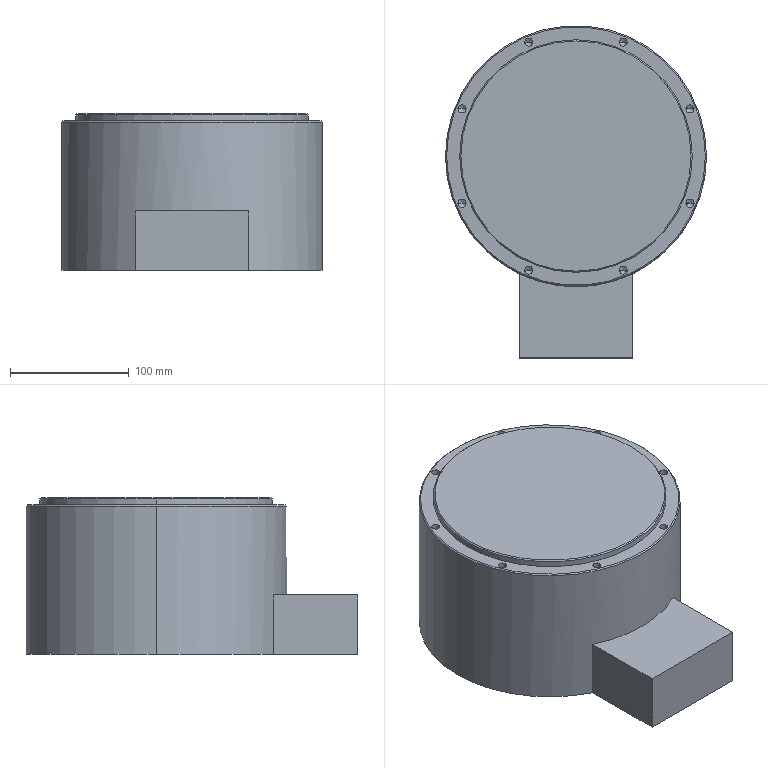Part | SolidWorks | features ICE 3, HoleWzd 2, Chamfer 1, Extrusion 1 | 1 solid | 51 faces | box 220 x 280 x 132 mm | volume 5270388 mm3 | cylinder 22 | cone 22 | plane 7 | commonest cylinder face diameters 6.8 x18 196 x2 220 x2
STEP:
#1=CARTESIAN_POINT('',(36.399,96.083,112.25));
#2=VERTEX_POINT('',#1);
#3=CARTESIAN_POINT('',(43.199,96.083,112.25));
#4=VERTEX_POINT('',#3);
#5=CARTESIAN_POINT('',(39.799,96.083,112.25));
#6=DIRECTION('',(0.,0.,1.));
#7=DIRECTION('',(1.,0.,0.));
#8=AXIS2_PLACEMENT_3D('',#5,#6,#7);
#9=CIRCLE('',#8,3.4);
#10=EDGE_CURVE('',#2,#4,#9,.T.);
#11=ORIENTED_EDGE('',*,*,#10,.F.);
#12=CARTESIAN_POINT('',(36.399,96.083,126.));
#13=VERTEX_POINT('',#12);
#14=CARTESIAN_POINT('',(36.399,96.083,132.));
#15=DIRECTION('',(0.,0.,1.));
#16=VECTOR('',#15,1000.);
#17=LINE('',#14,#16);
#18=EDGE_CURVE('',#2,#13,#17,.T.);
#19=ORIENTED_EDGE('',*,*,#18,.T.);
#20=CARTESIAN_POINT('',(43.199,96.083,126.));
#21=VERTEX_POINT('',#20);
#22=CARTESIAN_POINT('',(39.799,96.083,126.));
#23=DIRECTION('',(0.,0.,1.));
#24=DIRECTION('',(1.,0.,0.));
#25=AXIS2_PLACEMENT_3D('',#22,#23,#24);
#26=CIRCLE('',#25,3.4);
#27=EDGE_CURVE('',#13,#21,#26,.T.);
#28=ORIENTED_EDGE('',*,*,#27,.T.);
#29=CARTESIAN_POINT('',(43.199,96.083,132.));
#30=DIRECTION('',(0.,0.,1.));
#31=VECTOR('',#30,1000.);
#32=LINE('',#29,#31);
#33=EDGE_CURVE('',#4,#21,#32,.T.);
#34=ORIENTED_EDGE('',*,*,#33,.F.);
#35=EDGE_LOOP('',(#11,#19,#28,#34));
#36=FACE_OUTER_BOUND('',#35,.T.);
#37=CARTESIAN_POINT('',(39.799,96.083,132.));
#38=DIRECTION('',(0.,0.,1.));
#39=DIRECTION('',(1.,0.,0.));
#40=AXIS2_PLACEMENT_3D('',#37,#38,#39);
#41=CYLINDRICAL_SURFACE('',#40,3.4);
#42=ADVANCED_FACE('',(#36),#41,.F.);
#43=CARTESIAN_POINT('',(39.799,96.083,110.207));
#44=VERTEX_POINT('',#43);
#45=CARTESIAN_POINT('',(43.199,96.083,112.25));
#46=DIRECTION('',(0.8572,0.,0.515));
#47=VECTOR('',#46,1000.);
#48=LINE('',#45,#47);
#49=EDGE_CURVE('',#44,#4,#48,.T.);
#50=ORIENTED_EDGE('',*,*,#49,.F.);
#51=CARTESIAN_POINT('',(36.399,96.083,112.25));
#52=DIRECTION('',(-0.8572,0.,0.515));
#53=VECTOR('',#52,1000.);
#54=LINE('',#51,#53);
#55=EDGE_CURVE('',#44,#2,#54,.T.);
#56=ORIENTED_EDGE('',*,*,#55,.T.);
#57=ORIENTED_EDGE('',*,*,#10,.T.);
#58=EDGE_LOOP('',(#50,#56,#57));
#59=FACE_OUTER_BOUND('',#58,.T.);
#60=CARTESIAN_POINT('',(39.799,96.083,112.25));
#61=DIRECTION('',(0.,0.,1.));
#62=DIRECTION('',(1.,0.,0.));
#63=AXIS2_PLACEMENT_3D('',#60,#61,#62);
#64=CONICAL_SURFACE('',#63,3.4,1.03);
#65=ADVANCED_FACE('',(#59),#64,.F.);
#66=CARTESIAN_POINT('',(92.683,39.799,112.25));
#67=VERTEX_POINT('',#66);
#68=CARTESIAN_POINT('',(99.483,39.799,112.25));
#69=VERTEX_POINT('',#68);
#70=CARTESIAN_POINT('',(96.083,39.799,112.25));
#71=DIRECTION('',(0.,0.,1.));
#72=DIRECTION('',(1.,0.,0.));
#73=AXIS2_PLACEMENT_3D('',#70,#71,#72);
#74=CIRCLE('',#73,3.4);
#75=EDGE_CURVE('',#67,#69,#74,.T.);
#76=ORIENTED_EDGE('',*,*,#75,.F.);
#77=CARTESIAN_POINT('',(92.683,39.799,126.));
#78=VERTEX_POINT('',#77);
#79=CARTESIAN_POINT('',(92.683,39.799,132.));
#80=DIRECTION('',(0.,0.,1.));
#81=VECTOR('',#80,1000.);
#82=LINE('',#79,#81);
#83=EDGE_CURVE('',#67,#78,#82,.T.);
#84=ORIENTED_EDGE('',*,*,#83,.T.);
#85=CARTESIAN_POINT('',(99.483,39.799,126.));
#86=VERTEX_POINT('',#85);
#87=CARTESIAN_POINT('',(96.083,39.799,126.));
#88=DIRECTION('',(0.,0.,1.));
#89=DIRECTION('',(1.,0.,0.));
#90=AXIS2_PLACEMENT_3D('',#87,#88,#89);
#91=CIRCLE('',#90,3.4);
#92=EDGE_CURVE('',#78,#86,#91,.T.);
#93=ORIENTED_EDGE('',*,*,#92,.T.);
#94=CARTESIAN_POINT('',(99.483,39.799,132.));
#95=DIRECTION('',(0.,0.,1.));
#96=VECTOR('',#95,1000.);
#97=LINE('',#94,#96);
#98=EDGE_CURVE('',#69,#86,#97,.T.);
#99=ORIENTED_EDGE('',*,*,#98,.F.);
#100=EDGE_LOOP('',(#76,#84,#93,#99));
#101=FACE_OUTER_BOUND('',#100,.T.);
#102=CARTESIAN_POINT('',(96.083,39.799,132.));
#103=DIRECTION('',(0.,0.,1.));
#104=DIRECTION('',(1.,0.,0.));
#105=AXIS2_PLACEMENT_3D('',#102,#103,#104);
#106=CYLINDRICAL_SURFACE('',#105,3.4);
#107=ADVANCED_FACE('',(#101),#106,.F.);
#108=CARTESIAN_POINT('',(96.083,39.799,110.207));
#109=VERTEX_POINT('',#108);
#110=CARTESIAN_POINT('',(99.483,39.799,112.25));
#111=DIRECTION('',(0.8572,0.,0.515));
#112=VECTOR('',#111,1000.);
#113=LINE('',#110,#112);
#114=EDGE_CURVE('',#109,#69,#113,.T.);
#115=ORIENTED_EDGE('',*,*,#114,.F.);
#116=CARTESIAN_POINT('',(92.683,39.799,112.25));
#117=DIRECTION('',(-0.8572,0.,0.515));
#118=VECTOR('',#117,1000.);
#119=LINE('',#116,#118);
#120=EDGE_CURVE('',#109,#67,#119,.T.);
#121=ORIENTED_EDGE('',*,*,#120,.T.);
#122=ORIENTED_EDGE('',*,*,#75,.T.);
#123=EDGE_LOOP('',(#115,#121,#122));
#124=FACE_OUTER_BOUND('',#123,.T.);
#125=CARTESIAN_POINT('',(96.083,39.799,112.25));
#126=DIRECTION('',(0.,0.,1.));
#127=DIRECTION('',(1.,0.,0.));
#128=AXIS2_PLACEMENT_3D('',#125,#126,#127);
#129=CONICAL_SURFACE('',#128,3.4,1.03);
#130=ADVANCED_FACE('',(#124),#129,.F.);
#131=CARTESIAN_POINT('',(92.683,-39.799,112.25));
#132=VERTEX_POINT('',#131);
#133=CARTESIAN_POINT('',(99.483,-39.799,112.25));
#134=VERTEX_POINT('',#133);
#135=CARTESIAN_POINT('',(96.083,-39.799,112.25));
#136=DIRECTION('',(0.,0.,1.));
#137=DIRECTION('',(1.,0.,0.));
#138=AXIS2_PLACEMENT_3D('',#135,#136,#137);
#139=CIRCLE('',#138,3.4);
#140=EDGE_CURVE('',#132,#134,#139,.T.);
#141=ORIENTED_EDGE('',*,*,#140,.F.);
#142=CARTESIAN_POINT('',(92.683,-39.799,126.));
#143=VERTEX_POINT('',#142);
#144=CARTESIAN_POINT('',(92.683,-39.799,132.));
#145=DIRECTION('',(0.,0.,1.));
#146=VECTOR('',#145,1000.);
#147=LINE('',#144,#146);
#148=EDGE_CURVE('',#132,#143,#147,.T.);
#149=ORIENTED_EDGE('',*,*,#148,.T.);
#150=CARTESIAN_POINT('',(99.483,-39.799,126.));
#151=VERTEX_POINT('',#150);
#152=CARTESIAN_POINT('',(96.083,-39.799,126.));
#153=DIRECTION('',(0.,0.,1.));
#154=DIRECTION('',(1.,0.,0.));
#155=AXIS2_PLACEMENT_3D('',#152,#153,#154);
#156=CIRCLE('',#155,3.4);
#157=EDGE_CURVE('',#143,#151,#156,.T.);
#158=ORIENTED_EDGE('',*,*,#157,.T.);
#159=CARTESIAN_POINT('',(99.483,-39.799,132.));
#160=DIRECTION('',(0.,0.,1.));
#161=VECTOR('',#160,1000.);
#162=LINE('',#159,#161);
#163=EDGE_CURVE('',#134,#151,#162,.T.);
#164=ORIENTED_EDGE('',*,*,#163,.F.);
#165=EDGE_LOOP('',(#141,#149,#158,#164));
#166=FACE_OUTER_BOUND('',#165,.T.);
#167=CARTESIAN_POINT('',(96.083,-39.799,132.));
#168=DIRECTION('',(0.,0.,1.));
#169=DIRECTION('',(1.,0.,0.));
#170=AXIS2_PLACEMENT_3D('',#167,#168,#169);
#171=CYLINDRICAL_SURFACE('',#170,3.4);
#172=ADVANCED_FACE('',(#166),#171,.F.);
#173=CARTESIAN_POINT('',(96.083,-39.799,110.207));
#174=VERTEX_POINT('',#173);
#175=CARTESIAN_POINT('',(99.483,-39.799,112.25));
#176=DIRECTION('',(0.8572,0.,0.515));
#177=VECTOR('',#176,1000.);
#178=LINE('',#175,#177);
#179=EDGE_CURVE('',#174,#134,#178,.T.);
#180=ORIENTED_EDGE('',*,*,#179,.F.);
#181=CARTESIAN_POINT('',(92.683,-39.799,112.25));
#182=DIRECTION('',(-0.8572,0.,0.515));
#183=VECTOR('',#182,1000.);
#184=LINE('',#181,#183);
#185=EDGE_CURVE('',#174,#132,#184,.T.);
#186=ORIENTED_EDGE('',*,*,#185,.T.);
#187=ORIENTED_EDGE('',*,*,#140,.T.);
#188=EDGE_LOOP('',(#180,#186,#187));
#189=FACE_OUTER_BOUND('',#188,.T.);
#190=CARTESIAN_POINT('',(96.083,-39.799,112.25));
#191=DIRECTION('',(0.,0.,1.));
#192=DIRECTION('',(1.,0.,0.));
#193=AXIS2_PLACEMENT_3D('',#190,#191,#192);
#194=CONICAL_SURFACE('',#193,3.4,1.03);
#195=ADVANCED_FACE('',(#189),#194,.F.);
#196=CARTESIAN_POINT('',(36.399,-96.083,112.25));
#197=VERTEX_POINT('',#196);
#198=CARTESIAN_POINT('',(43.199,-96.083,112.25));
#199=VERTEX_POINT('',#198);
#200=CARTESIAN_POINT('',(39.799,-96.083,112.25));
#201=DIRECTION('',(0.,0.,1.));
#202=DIRECTION('',(1.,0.,0.));
#203=AXIS2_PLACEMENT_3D('',#200,#201,#202);
#204=CIRCLE('',#203,3.4);
#205=EDGE_CURVE('',#197,#199,#204,.T.);
#206=ORIENTED_EDGE('',*,*,#205,.F.);
#207=CARTESIAN_POINT('',(36.399,-96.083,126.));
#208=VERTEX_POINT('',#207);
#209=CARTESIAN_POINT('',(36.399,-96.083,132.));
#210=DIRECTION('',(0.,0.,1.));
#211=VECTOR('',#210,1000.);
#212=LINE('',#209,#211);
#213=EDGE_CURVE('',#197,#208,#212,.T.);
#214=ORIENTED_EDGE('',*,*,#213,.T.);
#215=CARTESIAN_POINT('',(43.199,-96.083,126.));
#216=VERTEX_POINT('',#215);
#217=CARTESIAN_POINT('',(39.799,-96.083,126.));
#218=DIRECTION('',(0.,0.,1.));
#219=DIRECTION('',(1.,0.,0.));
#220=AXIS2_PLACEMENT_3D('',#217,#218,#219);
#221=CIRCLE('',#220,3.4);
#222=EDGE_CURVE('',#208,#216,#221,.T.);
#223=ORIENTED_EDGE('',*,*,#222,.T.);
#224=CARTESIAN_POINT('',(43.199,-96.083,132.));
#225=DIRECTION('',(0.,0.,1.));
#226=VECTOR('',#225,1000.);
#227=LINE('',#224,#226);
#228=EDGE_CURVE('',#199,#216,#227,.T.);
#229=ORIENTED_EDGE('',*,*,#228,.F.);
#230=EDGE_LOOP('',(#206,#214,#223,#229));
#231=FACE_OUTER_BOUND('',#230,.T.);
#232=CARTESIAN_POINT('',(39.799,-96.083,132.));
#233=DIRECTION('',(0.,0.,1.));
#234=DIRECTION('',(1.,0.,0.));
#235=AXIS2_PLACEMENT_3D('',#232,#233,#234);
#236=CYLINDRICAL_SURFACE('',#235,3.4);
#237=ADVANCED_FACE('',(#231),#236,.F.);
#238=CARTESIAN_POINT('',(39.799,-96.083,110.207));
#239=VERTEX_POINT('',#238);
#240=CARTESIAN_POINT('',(43.199,-96.083,112.25));
#241=DIRECTION('',(0.8572,0.,0.515));
#242=VECTOR('',#241,1000.);
#243=LINE('',#240,#242);
#244=EDGE_CURVE('',#239,#199,#243,.T.);
#245=ORIENTED_EDGE('',*,*,#244,.F.);
#246=CARTESIAN_POINT('',(36.399,-96.083,112.25));
#247=DIRECTION('',(-0.8572,0.,0.515));
#248=VECTOR('',#247,1000.);
#249=LINE('',#246,#248);
#250=EDGE_CURVE('',#239,#197,#249,.T.);
#251=ORIENTED_EDGE('',*,*,#250,.T.);
#252=ORIENTED_EDGE('',*,*,#205,.T.);
#253=EDGE_LOOP('',(#245,#251,#252));
#254=FACE_OUTER_BOUND('',#253,.T.);
#255=CARTESIAN_POINT('',(39.799,-96.083,112.25));
#256=DIRECTION('',(0.,0.,1.));
#257=DIRECTION('',(1.,0.,0.));
#258=AXIS2_PLACEMENT_3D('',#255,#256,#257);
#259=CONICAL_SURFACE('',#258,3.4,1.03);
#260=ADVANCED_FACE('',(#254),#259,.F.);
#261=CARTESIAN_POINT('',(-43.199,-96.083,112.25));
#262=VERTEX_POINT('',#261);
#263=CARTESIAN_POINT('',(-36.399,-96.083,112.25));
#264=VERTEX_POINT('',#263);
#265=CARTESIAN_POINT('',(-39.799,-96.083,112.25));
#266=DIRECTION('',(0.,0.,1.));
#267=DIRECTION('',(1.,0.,0.));
#268=AXIS2_PLACEMENT_3D('',#265,#266,#267);
#269=CIRCLE('',#268,3.4);
#270=EDGE_CURVE('',#262,#264,#269,.T.);
#271=ORIENTED_EDGE('',*,*,#270,.F.);
#272=CARTESIAN_POINT('',(-43.199,-96.083,126.));
#273=VERTEX_POINT('',#272);
#274=CARTESIAN_POINT('',(-43.199,-96.083,132.));
#275=DIRECTION('',(0.,0.,1.));
#276=VECTOR('',#275,1000.);
#277=LINE('',#274,#276);
#278=EDGE_CURVE('',#262,#273,#277,.T.);
#279=ORIENTED_EDGE('',*,*,#278,.T.);
#280=CARTESIAN_POINT('',(-36.399,-96.083,126.));
#281=VERTEX_POINT('',#280);
#282=CARTESIAN_POINT('',(-39.799,-96.083,126.));
#283=DIRECTION('',(0.,0.,1.));
#284=DIRECTION('',(1.,0.,0.));
#285=AXIS2_PLACEMENT_3D('',#282,#283,#284);
#286=CIRCLE('',#285,3.4);
#287=EDGE_CURVE('',#273,#281,#286,.T.);
#288=ORIENTED_EDGE('',*,*,#287,.T.);
#289=CARTESIAN_POINT('',(-36.399,-96.083,132.));
#290=DIRECTION('',(0.,0.,1.));
#291=VECTOR('',#290,1000.);
#292=LINE('',#289,#291);
#293=EDGE_CURVE('',#264,#281,#292,.T.);
#294=ORIENTED_EDGE('',*,*,#293,.F.);
#295=EDGE_LOOP('',(#271,#279,#288,#294));
#296=FACE_OUTER_BOUND('',#295,.T.);
#297=CARTESIAN_POINT('',(-39.799,-96.083,132.));
#298=DIRECTION('',(0.,0.,1.));
#299=DIRECTION('',(1.,0.,0.));
#300=AXIS2_PLACEMENT_3D('',#297,#298,#299);
#301=CYLINDRICAL_SURFACE('',#300,3.4);
#302=ADVANCED_FACE('',(#296),#301,.F.);
#303=CARTESIAN_POINT('',(-39.799,-96.083,110.207));
#304=VERTEX_POINT('',#303);
#305=CARTESIAN_POINT('',(-36.399,-96.083,112.25));
#306=DIRECTION('',(0.8572,0.,0.515));
#307=VECTOR('',#306,1000.);
#308=LINE('',#305,#307);
#309=EDGE_CURVE('',#304,#264,#308,.T.);
#310=ORIENTED_EDGE('',*,*,#309,.F.);
#311=CARTESIAN_POINT('',(-43.199,-96.083,112.25));
#312=DIRECTION('',(-0.8572,0.,0.515));
#313=VECTOR('',#312,1000.);
#314=LINE('',#311,#313);
#315=EDGE_CURVE('',#304,#262,#314,.T.);
#316=ORIENTED_EDGE('',*,*,#315,.T.);
#317=ORIENTED_EDGE('',*,*,#270,.T.);
#318=EDGE_LOOP('',(#310,#316,#317));
#319=FACE_OUTER_BOUND('',#318,.T.);
#320=CARTESIAN_POINT('',(-39.799,-96.083,112.25));
#321=DIRECTION('',(0.,0.,1.));
#322=DIRECTION('',(1.,0.,0.));
#323=AXIS2_PLACEMENT_3D('',#320,#321,#322);
#324=CONICAL_SURFACE('',#323,3.4,1.03);
#325=ADVANCED_FACE('',(#319),#324,.F.);
#326=CARTESIAN_POINT('',(-99.483,-39.799,112.25));
#327=VERTEX_POINT('',#326);
#328=CARTESIAN_POINT('',(-92.683,-39.799,112.25));
#329=VERTEX_POINT('',#328);
#330=CARTESIAN_POINT('',(-96.083,-39.799,112.25));
#331=DIRECTION('',(0.,0.,1.));
#332=DIRECTION('',(1.,0.,0.));
#333=AXIS2_PLACEMENT_3D('',#330,#331,#332);
#334=CIRCLE('',#333,3.4);
#335=EDGE_CURVE('',#327,#329,#334,.T.);
#336=ORIENTED_EDGE('',*,*,#335,.F.);
#337=CARTESIAN_POINT('',(-99.483,-39.799,126.));
#338=VERTEX_POINT('',#337);
#339=CARTESIAN_POINT('',(-99.483,-39.799,132.));
#340=DIRECTION('',(0.,0.,1.));
#341=VECTOR('',#340,1000.);
#342=LINE('',#339,#341);
#343=EDGE_CURVE('',#327,#338,#342,.T.);
#344=ORIENTED_EDGE('',*,*,#343,.T.);
#345=CARTESIAN_POINT('',(-92.683,-39.799,126.));
#346=VERTEX_POINT('',#345);
#347=CARTESIAN_POINT('',(-96.083,-39.799,126.));
#348=DIRECTION('',(0.,0.,1.));
#349=DIRECTION('',(1.,0.,0.));
#350=AXIS2_PLACEMENT_3D('',#347,#348,#349);
#351=CIRCLE('',#350,3.4);
#352=EDGE_CURVE('',#338,#346,#351,.T.);
#353=ORIENTED_EDGE('',*,*,#352,.T.);
#354=CARTESIAN_POINT('',(-92.683,-39.799,132.));
#355=DIRECTION('',(0.,0.,1.));
#356=VECTOR('',#355,1000.);
#357=LINE('',#354,#356);
#358=EDGE_CURVE('',#329,#346,#357,.T.);
#359=ORIENTED_EDGE('',*,*,#358,.F.);
#360=EDGE_LOOP('',(#336,#344,#353,#359));
#361=FACE_OUTER_BOUND('',#360,.T.);
#362=CARTESIAN_POINT('',(-96.083,-39.799,132.));
#363=DIRECTION('',(0.,0.,1.));
#364=DIRECTION('',(1.,0.,0.));
#365=AXIS2_PLACEMENT_3D('',#362,#363,#364);
#366=CYLINDRICAL_SURFACE('',#365,3.4);
#367=ADVANCED_FACE('',(#361),#366,.F.);
#368=CARTESIAN_POINT('',(-96.083,-39.799,110.207));
#369=VERTEX_POINT('',#368);
#370=CARTESIAN_POINT('',(-92.683,-39.799,112.25));
#371=DIRECTION('',(0.8572,0.,0.515));
#372=VECTOR('',#371,1000.);
#373=LINE('',#370,#372);
#374=EDGE_CURVE('',#369,#329,#373,.T.);
#375=ORIENTED_EDGE('',*,*,#374,.F.);
#376=CARTESIAN_POINT('',(-99.483,-39.799,112.25));
#377=DIRECTION('',(-0.8572,0.,0.515));
#378=VECTOR('',#377,1000.);
#379=LINE('',#376,#378);
#380=EDGE_CURVE('',#369,#327,#379,.T.);
#381=ORIENTED_EDGE('',*,*,#380,.T.);
#382=ORIENTED_EDGE('',*,*,#335,.T.);
#383=EDGE_LOOP('',(#375,#381,#382));
#384=FACE_OUTER_BOUND('',#383,.T.);
#385=CARTESIAN_POINT('',(-96.083,-39.799,112.25));
#386=DIRECTION('',(0.,0.,1.));
#387=DIRECTION('',(1.,0.,0.));
#388=AXIS2_PLACEMENT_3D('',#385,#386,#387);
#389=CONICAL_SURFACE('',#388,3.4,1.03);
#390=ADVANCED_FACE('',(#384),#389,.F.);
#391=CARTESIAN_POINT('',(-99.483,39.799,112.25));
#392=VERTEX_POINT('',#391);
#393=CARTESIAN_POINT('',(-92.683,39.799,112.25));
#394=VERTEX_POINT('',#393);
#395=CARTESIAN_POINT('',(-96.083,39.799,112.25));
#396=DIRECTION('',(0.,0.,1.));
#397=DIRECTION('',(1.,0.,0.));
#398=AXIS2_PLACEMENT_3D('',#395,#396,#397);
#399=CIRCLE('',#398,3.4);
#400=EDGE_CURVE('',#392,#394,#399,.T.);
#401=ORIENTED_EDGE('',*,*,#400,.F.);
#402=CARTESIAN_POINT('',(-99.483,39.799,126.));
#403=VERTEX_POINT('',#402);
#404=CARTESIAN_POINT('',(-99.483,39.799,132.));
#405=DIRECTION('',(0.,0.,1.));
#406=VECTOR('',#405,1000.);
#407=LINE('',#404,#406);
#408=EDGE_CURVE('',#392,#403,#407,.T.);
#409=ORIENTED_EDGE('',*,*,#408,.T.);
#410=CARTESIAN_POINT('',(-92.683,39.799,126.));
#411=VERTEX_POINT('',#410);
#412=CARTESIAN_POINT('',(-96.083,39.799,126.));
#413=DIRECTION('',(0.,0.,1.));
#414=DIRECTION('',(1.,0.,0.));
#415=AXIS2_PLACEMENT_3D('',#412,#413,#414);
#416=CIRCLE('',#415,3.4);
#417=EDGE_CURVE('',#403,#411,#416,.T.);
#418=ORIENTED_EDGE('',*,*,#417,.T.);
#419=CARTESIAN_POINT('',(-92.683,39.799,132.));
#420=DIRECTION('',(0.,0.,1.));
#421=VECTOR('',#420,1000.);
#422=LINE('',#419,#421);
#423=EDGE_CURVE('',#394,#411,#422,.T.);
#424=ORIENTED_EDGE('',*,*,#423,.F.);
#425=EDGE_LOOP('',(#401,#409,#418,#424));
#426=FACE_OUTER_BOUND('',#425,.T.);
#427=CARTESIAN_POINT('',(-96.083,39.799,132.));
#428=DIRECTION('',(0.,0.,1.));
#429=DIRECTION('',(1.,0.,0.));
#430=AXIS2_PLACEMENT_3D('',#427,#428,#429);
#431=CYLINDRICAL_SURFACE('',#430,3.4);
#432=ADVANCED_FACE('',(#426),#431,.F.);
#433=CARTESIAN_POINT('',(-96.083,39.799,110.207));
#434=VERTEX_POINT('',#433);
#435=CARTESIAN_POINT('',(-92.683,39.799,112.25));
#436=DIRECTION('',(0.8572,0.,0.515));
#437=VECTOR('',#436,1000.);
#438=LINE('',#435,#437);
#439=EDGE_CURVE('',#434,#394,#438,.T.);
#440=ORIENTED_EDGE('',*,*,#439,.F.);
#441=CARTESIAN_POINT('',(-99.483,39.799,112.25));
#442=DIRECTION('',(-0.8572,0.,0.515));
#443=VECTOR('',#442,1000.);
#444=LINE('',#441,#443);
#445=EDGE_CURVE('',#434,#392,#444,.T.);
#446=ORIENTED_EDGE('',*,*,#445,.T.);
#447=ORIENTED_EDGE('',*,*,#400,.T.);
#448=EDGE_LOOP('',(#440,#446,#447));
#449=FACE_OUTER_BOUND('',#448,.T.);
#450=CARTESIAN_POINT('',(-96.083,39.799,112.25));
#451=DIRECTION('',(0.,0.,1.));
#452=DIRECTION('',(1.,0.,0.));
#453=AXIS2_PLACEMENT_3D('',#450,#451,#452);
#454=CONICAL_SURFACE('',#453,3.4,1.03);
#455=ADVANCED_FACE('',(#449),#454,.F.);
#456=CARTESIAN_POINT('',(-43.199,96.083,112.25));
#457=VERTEX_POINT('',#456);
#458=CARTESIAN_POINT('',(-36.399,96.083,112.25));
#459=VERTEX_POINT('',#458);
#460=CARTESIAN_POINT('',(-39.799,96.083,112.25));
#461=DIRECTION('',(0.,0.,1.));
#462=DIRECTION('',(1.,0.,0.));
#463=AXIS2_PLACEMENT_3D('',#460,#461,#462);
#464=CIRCLE('',#463,3.4);
#465=EDGE_CURVE('',#457,#459,#464,.T.);
#466=ORIENTED_EDGE('',*,*,#465,.F.);
#467=CARTESIAN_POINT('',(-43.199,96.083,126.));
#468=VERTEX_POINT('',#467);
#469=CARTESIAN_POINT('',(-43.199,96.083,132.));
#470=DIRECTION('',(0.,0.,1.));
#471=VECTOR('',#470,1000.);
#472=LINE('',#469,#471);
#473=EDGE_CURVE('',#457,#468,#472,.T.);
#474=ORIENTED_EDGE('',*,*,#473,.T.);
#475=CARTESIAN_POINT('',(-36.399,96.083,126.));
#476=VERTEX_POINT('',#475);
#477=CARTESIAN_POINT('',(-39.799,96.083,126.));
#478=DIRECTION('',(0.,0.,1.));
#479=DIRECTION('',(1.,0.,0.));
#480=AXIS2_PLACEMENT_3D('',#477,#478,#479);
#481=CIRCLE('',#480,3.4);
#482=EDGE_CURVE('',#468,#476,#481,.T.);
#483=ORIENTED_EDGE('',*,*,#482,.T.);
#484=CARTESIAN_POINT('',(-36.399,96.083,132.));
#485=DIRECTION('',(0.,0.,1.));
#486=VECTOR('',#485,1000.);
#487=LINE('',#484,#486);
#488=EDGE_CURVE('',#459,#476,#487,.T.);
#489=ORIENTED_EDGE('',*,*,#488,.F.);
#490=EDGE_LOOP('',(#466,#474,#483,#489));
#491=FACE_OUTER_BOUND('',#490,.T.);
#492=CARTESIAN_POINT('',(-39.799,96.083,132.));
#493=DIRECTION('',(0.,0.,1.));
#494=DIRECTION('',(1.,0.,0.));
#495=AXIS2_PLACEMENT_3D('',#492,#493,#494);
#496=CYLINDRICAL_SURFACE('',#495,3.4);
#497=ADVANCED_FACE('',(#491),#496,.F.);
#498=CARTESIAN_POINT('',(-39.799,96.083,110.207));
#499=VERTEX_POINT('',#498);
#500=CARTESIAN_POINT('',(-36.399,96.083,112.25));
#501=DIRECTION('',(0.8572,0.,0.515));
#502=VECTOR('',#501,1000.);
#503=LINE('',#500,#502);
#504=EDGE_CURVE('',#499,#459,#503,.T.);
#505=ORIENTED_EDGE('',*,*,#504,.F.);
#506=CARTESIAN_POINT('',(-43.199,96.083,112.25));
#507=DIRECTION('',(-0.8572,0.,0.515));
#508=VECTOR('',#507,1000.);
#509=LINE('',#506,#508);
#510=EDGE_CURVE('',#499,#457,#509,.T.);
#511=ORIENTED_EDGE('',*,*,#510,.T.);
#512=ORIENTED_EDGE('',*,*,#465,.T.);
#513=EDGE_LOOP('',(#505,#511,#512));
#514=FACE_OUTER_BOUND('',#513,.T.);
#515=CARTESIAN_POINT('',(-39.799,96.083,112.25));
#516=DIRECTION('',(0.,0.,1.));
#517=DIRECTION('',(1.,0.,0.));
#518=AXIS2_PLACEMENT_3D('',#515,#516,#517);
#519=CONICAL_SURFACE('',#518,3.4,1.03);
#520=ADVANCED_FACE('',(#514),#519,.F.);
#521=CARTESIAN_POINT('',(3.4,-115.,19.75));
#522=VERTEX_POINT('',#521);
#523=CARTESIAN_POINT('',(-3.4,-115.,19.75));
#524=VERTEX_POINT('',#523);
#525=CARTESIAN_POINT('',(0.,-115.,19.75));
#526=DIRECTION('',(0.,0.,-1.));
#527=DIRECTION('',(-1.,0.,0.));
#528=AXIS2_PLACEMENT_3D('',#525,#526,#527);
#529=CIRCLE('',#528,3.4);
#530=EDGE_CURVE('',#522,#524,#529,.T.);
#531=ORIENTED_EDGE('',*,*,#530,.F.);
#532=CARTESIAN_POINT('',(3.4,-115.,0.));
#533=VERTEX_POINT('',#532);
#534=CARTESIAN_POINT('',(3.4,-115.,0.));
#535=DIRECTION('',(0.,0.,-1.));
#536=VECTOR('',#535,1000.);
#537=LINE('',#534,#536);
#538=EDGE_CURVE('',#522,#533,#537,.T.);
#539=ORIENTED_EDGE('',*,*,#538,.T.);
#540=CARTESIAN_POINT('',(-3.4,-115.,0.));
#541=VERTEX_POINT('',#540);
#542=CARTESIAN_POINT('',(0.,-115.,0.));
#543=DIRECTION('',(0.,0.,-1.));
#544=DIRECTION('',(-1.,0.,0.));
#545=AXIS2_PLACEMENT_3D('',#542,#543,#544);
#546=CIRCLE('',#545,3.4);
#547=EDGE_CURVE('',#533,#541,#546,.T.);
#548=ORIENTED_EDGE('',*,*,#547,.T.);
#549=CARTESIAN_POINT('',(-3.4,-115.,0.));
#550=DIRECTION('',(0.,0.,-1.));
#551=VECTOR('',#550,1000.);
#552=LINE('',#549,#551);
#553=EDGE_CURVE('',#524,#541,#552,.T.);
#554=ORIENTED_EDGE('',*,*,#553,.F.);
#555=EDGE_LOOP('',(#531,#539,#548,#554));
#556=FACE_OUTER_BOUND('',#555,.T.);
#557=CARTESIAN_POINT('',(0.,-115.,0.));
#558=DIRECTION('',(0.,0.,-1.));
#559=DIRECTION('',(-1.,0.,0.));
#560=AXIS2_PLACEMENT_3D('',#557,#558,#559);
#561=CYLINDRICAL_SURFACE('',#560,3.4);
#562=ADVANCED_FACE('',(#556),#561,.F.);
#563=CARTESIAN_POINT('',(0.,-115.,21.793));
#564=VERTEX_POINT('',#563);
#565=CARTESIAN_POINT('',(-3.4,-115.,19.75));
#566=DIRECTION('',(-0.8572,0.,-0.515));
#567=VECTOR('',#566,1000.);
#568=LINE('',#565,#567);
#569=EDGE_CURVE('',#564,#524,#568,.T.);
#570=ORIENTED_EDGE('',*,*,#569,.F.);
#571=CARTESIAN_POINT('',(3.4,-115.,19.75));
#572=DIRECTION('',(0.8572,0.,-0.515));
#573=VECTOR('',#572,1000.);
#574=LINE('',#571,#573);
#575=EDGE_CURVE('',#564,#522,#574,.T.);
#576=ORIENTED_EDGE('',*,*,#575,.T.);
#577=ORIENTED_EDGE('',*,*,#530,.T.);
#578=EDGE_LOOP('',(#570,#576,#577));
#579=FACE_OUTER_BOUND('',#578,.T.);
#580=CARTESIAN_POINT('',(0.,-115.,19.75));
#581=DIRECTION('',(0.,0.,-1.));
#582=DIRECTION('',(-1.,0.,0.));
#583=AXIS2_PLACEMENT_3D('',#580,#581,#582);
#584=CONICAL_SURFACE('',#583,3.4,1.03);
#585=ADVANCED_FACE('',(#579),#584,.F.);
#586=CARTESIAN_POINT('',(109.,0.,126.));
#587=VERTEX_POINT('',#586);
#588=CARTESIAN_POINT('',(-109.,0.,126.));
#589=VERTEX_POINT('',#588);
#590=CARTESIAN_POINT('',(0.,0.,126.));
#591=DIRECTION('',(0.,0.,1.));
#592=DIRECTION('',(1.,0.,0.));
#593=AXIS2_PLACEMENT_3D('',#590,#591,#592);
#594=CIRCLE('',#593,109.);
#595=EDGE_CURVE('',#587,#589,#594,.T.);
#596=ORIENTED_EDGE('',*,*,#595,.F.);
#597=CARTESIAN_POINT('',(110.,0.,125.));
#598=VERTEX_POINT('',#597);
#599=CARTESIAN_POINT('',(109.,0.,126.));
#600=DIRECTION('',(0.7071,0.,-0.7071));
#601=VECTOR('',#600,1000.);
#602=LINE('',#599,#601);
#603=EDGE_CURVE('',#587,#598,#602,.T.);
#604=ORIENTED_EDGE('',*,*,#603,.T.);
#605=CARTESIAN_POINT('',(-110.,0.,125.));
#606=VERTEX_POINT('',#605);
#607=CARTESIAN_POINT('',(0.,0.,125.));
#608=DIRECTION('',(0.,0.,-1.));
#609=DIRECTION('',(1.,0.,0.));
#610=AXIS2_PLACEMENT_3D('',#607,#608,#609);
#611=CIRCLE('',#610,110.);
#612=EDGE_CURVE('',#606,#598,#611,.T.);
#613=ORIENTED_EDGE('',*,*,#612,.F.);
#614=CARTESIAN_POINT('',(-109.,0.,126.));
#615=DIRECTION('',(-0.7071,0.,-0.7071));
#616=VECTOR('',#615,1000.);
#617=LINE('',#614,#616);
#618=EDGE_CURVE('',#589,#606,#617,.T.);
#619=ORIENTED_EDGE('',*,*,#618,.F.);
#620=EDGE_LOOP('',(#596,#604,#613,#619));
#621=FACE_OUTER_BOUND('',#620,.T.);
#622=CARTESIAN_POINT('',(0.,0.,126.));
#623=DIRECTION('',(0.,0.,-1.));
#624=DIRECTION('',(-1.,0.,0.));
#625=AXIS2_PLACEMENT_3D('',#622,#623,#624);
#626=CONICAL_SURFACE('',#625,109.,0.7854);
#627=ADVANCED_FACE('',(#621),#626,.T.);
#628=CARTESIAN_POINT('',(97.,0.,132.));
#629=VERTEX_POINT('',#628);
#630=CARTESIAN_POINT('',(-97.,0.,132.));
#631=VERTEX_POINT('',#630);
#632=CARTESIAN_POINT('',(0.,0.,132.));
#633=DIRECTION('',(0.,0.,1.));
#634=DIRECTION('',(1.,0.,0.));
#635=AXIS2_PLACEMENT_3D('',#632,#633,#634);
#636=CIRCLE('',#635,97.);
#637=EDGE_CURVE('',#629,#631,#636,.T.);
#638=ORIENTED_EDGE('',*,*,#637,.F.);
#639=CARTESIAN_POINT('',(98.,0.,131.));
#640=VERTEX_POINT('',#639);
#641=CARTESIAN_POINT('',(97.,0.,132.));
#642=DIRECTION('',(0.7071,0.,-0.7071));
#643=VECTOR('',#642,1000.);
#644=LINE('',#641,#643);
#645=EDGE_CURVE('',#629,#640,#644,.T.);
#646=ORIENTED_EDGE('',*,*,#645,.T.);
#647=CARTESIAN_POINT('',(-98.,0.,131.));
#648=VERTEX_POINT('',#647);
#649=CARTESIAN_POINT('',(0.,0.,131.));
#650=DIRECTION('',(0.,0.,-1.));
#651=DIRECTION('',(1.,0.,0.));
#652=AXIS2_PLACEMENT_3D('',#649,#650,#651);
#653=CIRCLE('',#652,98.);
#654=EDGE_CURVE('',#648,#640,#653,.T.);
#655=ORIENTED_EDGE('',*,*,#654,.F.);
#656=CARTESIAN_POINT('',(-97.,0.,132.));
#657=DIRECTION('',(-0.7071,0.,-0.7071));
#658=VECTOR('',#657,1000.);
#659=LINE('',#656,#658);
#660=EDGE_CURVE('',#631,#648,#659,.T.);
#661=ORIENTED_EDGE('',*,*,#660,.F.);
#662=EDGE_LOOP('',(#638,#646,#655,#661));
#663=FACE_OUTER_BOUND('',#662,.T.);
#664=CARTESIAN_POINT('',(0.,0.,132.));
#665=DIRECTION('',(0.,0.,-1.));
#666=DIRECTION('',(-1.,0.,0.));
#667=AXIS2_PLACEMENT_3D('',#664,#665,#666);
#668=CONICAL_SURFACE('',#667,97.,0.7854);
#669=ADVANCED_FACE('',(#663),#668,.T.);
#670=ORIENTED_EDGE('',*,*,#654,.T.);
#671=CARTESIAN_POINT('',(98.,0.,126.));
#672=VERTEX_POINT('',#671);
#673=CARTESIAN_POINT('',(98.,0.,132.));
#674=DIRECTION('',(0.,0.,-1.));
#675=VECTOR('',#674,1000.);
#676=LINE('',#673,#675);
#677=EDGE_CURVE('',#640,#672,#676,.T.);
#678=ORIENTED_EDGE('',*,*,#677,.T.);
#679=CARTESIAN_POINT('',(-98.,0.,126.));
#680=VERTEX_POINT('',#679);
#681=CARTESIAN_POINT('',(0.,0.,126.));
#682=DIRECTION('',(0.,0.,1.));
#683=DIRECTION('',(1.,0.,0.));
#684=AXIS2_PLACEMENT_3D('',#681,#682,#683);
#685=CIRCLE('',#684,98.);
#686=EDGE_CURVE('',#672,#680,#685,.T.);
#687=ORIENTED_EDGE('',*,*,#686,.T.);
#688=CARTESIAN_POINT('',(-98.,0.,132.));
#689=DIRECTION('',(0.,0.,-1.));
#690=VECTOR('',#689,1000.);
#691=LINE('',#688,#690);
#692=EDGE_CURVE('',#648,#680,#691,.T.);
#693=ORIENTED_EDGE('',*,*,#692,.F.);
#694=EDGE_LOOP('',(#670,#678,#687,#693));
#695=FACE_OUTER_BOUND('',#694,.T.);
#696=CARTESIAN_POINT('',(0.,0.,132.));
#697=DIRECTION('',(0.,0.,-1.));
#698=DIRECTION('',(-1.,0.,0.));
#699=AXIS2_PLACEMENT_3D('',#696,#697,#698);
#700=CYLINDRICAL_SURFACE('',#699,98.);
#701=ADVANCED_FACE('',(#695),#700,.T.);
#702=ORIENTED_EDGE('',*,*,#612,.T.);
#703=CARTESIAN_POINT('',(110.,0.,0.));
#704=VERTEX_POINT('',#703);
#705=CARTESIAN_POINT('',(110.,0.,126.));
#706=DIRECTION('',(0.,0.,-1.));
#707=VECTOR('',#706,1000.);
#708=LINE('',#705,#707);
#709=EDGE_CURVE('',#598,#704,#708,.T.);
#710=ORIENTED_EDGE('',*,*,#709,.T.);
#711=CARTESIAN_POINT('',(-110.,0.,0.));
#712=VERTEX_POINT('',#711);
#713=CARTESIAN_POINT('',(0.,0.,0.));
#714=DIRECTION('',(0.,0.,1.));
#715=DIRECTION('',(1.,0.,0.));
#716=AXIS2_PLACEMENT_3D('',#713,#714,#715);
#717=CIRCLE('',#716,110.);
#718=EDGE_CURVE('',#704,#712,#717,.T.);
#719=ORIENTED_EDGE('',*,*,#718,.T.);
#720=CARTESIAN_POINT('',(-110.,0.,126.));
#721=DIRECTION('',(0.,0.,-1.));
#722=VECTOR('',#721,1000.);
#723=LINE('',#720,#722);
#724=EDGE_CURVE('',#606,#712,#723,.T.);
#725=ORIENTED_EDGE('',*,*,#724,.F.);
#726=EDGE_LOOP('',(#702,#710,#719,#725));
#727=FACE_OUTER_BOUND('',#726,.T.);
#728=CARTESIAN_POINT('',(0.,0.,126.));
#729=DIRECTION('',(0.,0.,-1.));
#730=DIRECTION('',(-1.,0.,0.));
#731=AXIS2_PLACEMENT_3D('',#728,#729,#730);
#732=CYLINDRICAL_SURFACE('',#731,110.);
#733=ADVANCED_FACE('',(#727),#732,.T.);
#734=ORIENTED_EDGE('',*,*,#709,.F.);
#735=CARTESIAN_POINT('',(0.,0.,125.));
#736=DIRECTION('',(0.,0.,-1.));
#737=DIRECTION('',(1.,0.,0.));
#738=AXIS2_PLACEMENT_3D('',#735,#736,#737);
#739=CIRCLE('',#738,110.);
#740=EDGE_CURVE('',#598,#606,#739,.T.);
#741=ORIENTED_EDGE('',*,*,#740,.T.);
#742=ORIENTED_EDGE('',*,*,#724,.T.);
#743=CARTESIAN_POINT('',(-48.,-98.975,0.));
#744=VERTEX_POINT('',#743);
#745=CARTESIAN_POINT('',(0.,0.,0.));
#746=DIRECTION('',(0.,0.,1.));
#747=DIRECTION('',(1.,0.,0.));
#748=AXIS2_PLACEMENT_3D('',#745,#746,#747);
#749=CIRCLE('',#748,110.);
#750=EDGE_CURVE('',#712,#744,#749,.T.);
#751=ORIENTED_EDGE('',*,*,#750,.T.);
#752=CARTESIAN_POINT('',(-48.,-98.975,50.));
#753=VERTEX_POINT('',#752);
#754=CARTESIAN_POINT('',(-48.,-98.975,50.));
#755=DIRECTION('',(0.,0.,-1.));
#756=VECTOR('',#755,1000.);
#757=LINE('',#754,#756);
#758=EDGE_CURVE('',#753,#744,#757,.T.);
#759=ORIENTED_EDGE('',*,*,#758,.F.);
#760=CARTESIAN_POINT('',(48.,-98.975,50.));
#761=VERTEX_POINT('',#760);
#762=CARTESIAN_POINT('',(0.,0.,50.));
#763=DIRECTION('',(0.,0.,-1.));
#764=DIRECTION('',(-1.,0.,0.));
#765=AXIS2_PLACEMENT_3D('',#762,#763,#764);
#766=CIRCLE('',#765,110.);
#767=EDGE_CURVE('',#761,#753,#766,.T.);
#768=ORIENTED_EDGE('',*,*,#767,.F.);
#769=CARTESIAN_POINT('',(48.,-98.975,0.));
#770=VERTEX_POINT('',#769);
#771=CARTESIAN_POINT('',(48.,-98.975,50.));
#772=DIRECTION('',(0.,0.,-1.));
#773=VECTOR('',#772,1000.);
#774=LINE('',#771,#773);
#775=EDGE_CURVE('',#761,#770,#774,.T.);
#776=ORIENTED_EDGE('',*,*,#775,.T.);
#777=CARTESIAN_POINT('',(0.,0.,0.));
#778=DIRECTION('',(0.,0.,1.));
#779=DIRECTION('',(1.,0.,0.));
#780=AXIS2_PLACEMENT_3D('',#777,#778,#779);
#781=CIRCLE('',#780,110.);
#782=EDGE_CURVE('',#770,#704,#781,.T.);
#783=ORIENTED_EDGE('',*,*,#782,.T.);
#784=EDGE_LOOP('',(#734,#741,#742,#751,#759,#768,#776,#783));
#785=FACE_OUTER_BOUND('',#784,.T.);
#786=CARTESIAN_POINT('',(0.,0.,126.));
#787=DIRECTION('',(0.,0.,-1.));
#788=DIRECTION('',(-1.,0.,0.));
#789=AXIS2_PLACEMENT_3D('',#786,#787,#788);
#790=CYLINDRICAL_SURFACE('',#789,110.);
#791=ADVANCED_FACE('',(#785),#790,.T.);
#792=CARTESIAN_POINT('',(39.799,96.083,126.));
#793=DIRECTION('',(0.,0.,1.));
#794=DIRECTION('',(1.,0.,0.));
#795=AXIS2_PLACEMENT_3D('',#792,#793,#794);
#796=CIRCLE('',#795,3.4);
#797=EDGE_CURVE('',#21,#13,#796,.T.);
#798=ORIENTED_EDGE('',*,*,#797,.F.);
#799=ORIENTED_EDGE('',*,*,#27,.F.);
#800=EDGE_LOOP('',(#798,#799));
#801=FACE_BOUND('',#800,.T.);
#802=CARTESIAN_POINT('',(96.083,39.799,126.));
#803=DIRECTION('',(0.,0.,1.));
#804=DIRECTION('',(1.,0.,0.));
#805=AXIS2_PLACEMENT_3D('',#802,#803,#804);
#806=CIRCLE('',#805,3.4);
#807=EDGE_CURVE('',#86,#78,#806,.T.);
#808=ORIENTED_EDGE('',*,*,#807,.F.);
#809=ORIENTED_EDGE('',*,*,#92,.F.);
#810=EDGE_LOOP('',(#808,#809));
#811=FACE_BOUND('',#810,.T.);
#812=CARTESIAN_POINT('',(96.083,-39.799,126.));
#813=DIRECTION('',(0.,0.,1.));
#814=DIRECTION('',(1.,0.,0.));
#815=AXIS2_PLACEMENT_3D('',#812,#813,#814);
#816=CIRCLE('',#815,3.4);
#817=EDGE_CURVE('',#151,#143,#816,.T.);
#818=ORIENTED_EDGE('',*,*,#817,.F.);
#819=ORIENTED_EDGE('',*,*,#157,.F.);
#820=EDGE_LOOP('',(#818,#819));
#821=FACE_BOUND('',#820,.T.);
#822=CARTESIAN_POINT('',(39.799,-96.083,126.));
#823=DIRECTION('',(0.,0.,1.));
#824=DIRECTION('',(1.,0.,0.));
#825=AXIS2_PLACEMENT_3D('',#822,#823,#824);
#826=CIRCLE('',#825,3.4);
#827=EDGE_CURVE('',#216,#208,#826,.T.);
#828=ORIENTED_EDGE('',*,*,#827,.F.);
#829=ORIENTED_EDGE('',*,*,#222,.F.);
#830=EDGE_LOOP('',(#828,#829));
#831=FACE_BOUND('',#830,.T.);
#832=CARTESIAN_POINT('',(-39.799,-96.083,126.));
#833=DIRECTION('',(0.,0.,1.));
#834=DIRECTION('',(1.,0.,0.));
#835=AXIS2_PLACEMENT_3D('',#832,#833,#834);
#836=CIRCLE('',#835,3.4);
#837=EDGE_CURVE('',#281,#273,#836,.T.);
#838=ORIENTED_EDGE('',*,*,#837,.F.);
#839=ORIENTED_EDGE('',*,*,#287,.F.);
#840=EDGE_LOOP('',(#838,#839));
#841=FACE_BOUND('',#840,.T.);
#842=CARTESIAN_POINT('',(-96.083,-39.799,126.));
#843=DIRECTION('',(0.,0.,1.));
#844=DIRECTION('',(1.,0.,0.));
#845=AXIS2_PLACEMENT_3D('',#842,#843,#844);
#846=CIRCLE('',#845,3.4);
#847=EDGE_CURVE('',#346,#338,#846,.T.);
#848=ORIENTED_EDGE('',*,*,#847,.F.);
#849=ORIENTED_EDGE('',*,*,#352,.F.);
#850=EDGE_LOOP('',(#848,#849));
#851=FACE_BOUND('',#850,.T.);
#852=CARTESIAN_POINT('',(-96.083,39.799,126.));
#853=DIRECTION('',(0.,0.,1.));
#854=DIRECTION('',(1.,0.,0.));
#855=AXIS2_PLACEMENT_3D('',#852,#853,#854);
#856=CIRCLE('',#855,3.4);
#857=EDGE_CURVE('',#411,#403,#856,.T.);
#858=ORIENTED_EDGE('',*,*,#857,.F.);
#859=ORIENTED_EDGE('',*,*,#417,.F.);
#860=EDGE_LOOP('',(#858,#859));
#861=FACE_BOUND('',#860,.T.);
#862=CARTESIAN_POINT('',(-39.799,96.083,126.));
#863=DIRECTION('',(0.,0.,1.));
#864=DIRECTION('',(1.,0.,0.));
#865=AXIS2_PLACEMENT_3D('',#862,#863,#864);
#866=CIRCLE('',#865,3.4);
#867=EDGE_CURVE('',#476,#468,#866,.T.);
#868=ORIENTED_EDGE('',*,*,#867,.F.);
#869=ORIENTED_EDGE('',*,*,#482,.F.);
#870=EDGE_LOOP('',(#868,#869));
#871=FACE_BOUND('',#870,.T.);
#872=CARTESIAN_POINT('',(0.,0.,126.));
#873=DIRECTION('',(0.,0.,1.));
#874=DIRECTION('',(1.,0.,0.));
#875=AXIS2_PLACEMENT_3D('',#872,#873,#874);
#876=CIRCLE('',#875,109.);
#877=EDGE_CURVE('',#589,#587,#876,.T.);
#878=ORIENTED_EDGE('',*,*,#877,.T.);
#879=ORIENTED_EDGE('',*,*,#595,.T.);
#880=EDGE_LOOP('',(#878,#879));
#881=FACE_OUTER_BOUND('',#880,.T.);
#882=CARTESIAN_POINT('',(0.,0.,126.));
#883=DIRECTION('',(0.,0.,1.));
#884=DIRECTION('',(1.,0.,0.));
#885=AXIS2_PLACEMENT_3D('',#882,#883,#884);
#886=CIRCLE('',#885,98.);
#887=EDGE_CURVE('',#680,#672,#886,.T.);
#888=ORIENTED_EDGE('',*,*,#887,.F.);
#889=ORIENTED_EDGE('',*,*,#686,.F.);
#890=EDGE_LOOP('',(#888,#889));
#891=FACE_BOUND('',#890,.T.);
#892=CARTESIAN_POINT('',(0.,0.,126.));
#893=DIRECTION('',(0.,0.,1.));
#894=DIRECTION('',(1.,0.,0.));
#895=AXIS2_PLACEMENT_3D('',#892,#893,#894);
#896=PLANE('',#895);
#897=ADVANCED_FACE('',(#801,#811,#821,#831,#841,#851,#861,#871,#881,#891),#896,.T.);
#898=CARTESIAN_POINT('',(0.,-115.,0.));
#899=DIRECTION('',(0.,0.,-1.));
#900=DIRECTION('',(-1.,0.,0.));
#901=AXIS2_PLACEMENT_3D('',#898,#899,#900);
#902=CIRCLE('',#901,3.4);
#903=EDGE_CURVE('',#541,#533,#902,.T.);
#904=ORIENTED_EDGE('',*,*,#903,.F.);
#905=ORIENTED_EDGE('',*,*,#547,.F.);
#906=EDGE_LOOP('',(#904,#905));
#907=FACE_BOUND('',#906,.T.);
#908=ORIENTED_EDGE('',*,*,#782,.F.);
#909=CARTESIAN_POINT('',(48.,-170.,0.));
#910=VERTEX_POINT('',#909);
#911=CARTESIAN_POINT('',(48.,-98.975,0.));
#912=DIRECTION('',(0.,-1.,0.));
#913=VECTOR('',#912,1000.);
#914=LINE('',#911,#913);
#915=EDGE_CURVE('',#770,#910,#914,.T.);
#916=ORIENTED_EDGE('',*,*,#915,.T.);
#917=CARTESIAN_POINT('',(-48.,-170.,0.));
#918=VERTEX_POINT('',#917);
#919=CARTESIAN_POINT('',(48.,-170.,0.));
#920=DIRECTION('',(-1.,0.,0.));
#921=VECTOR('',#920,1000.);
#922=LINE('',#919,#921);
#923=EDGE_CURVE('',#910,#918,#922,.T.);
#924=ORIENTED_EDGE('',*,*,#923,.T.);
#925=CARTESIAN_POINT('',(-48.,-98.975,0.));
#926=DIRECTION('',(0.,1.,0.));
#927=VECTOR('',#926,1000.);
#928=LINE('',#925,#927);
#929=EDGE_CURVE('',#918,#744,#928,.T.);
#930=ORIENTED_EDGE('',*,*,#929,.T.);
#931=ORIENTED_EDGE('',*,*,#750,.F.);
#932=ORIENTED_EDGE('',*,*,#718,.F.);
#933=EDGE_LOOP('',(#908,#916,#924,#930,#931,#932));
#934=FACE_OUTER_BOUND('',#933,.T.);
#935=CARTESIAN_POINT('',(0.,0.,0.));
#936=DIRECTION('',(0.,0.,1.));
#937=DIRECTION('',(1.,0.,0.));
#938=AXIS2_PLACEMENT_3D('',#935,#936,#937);
#939=PLANE('',#938);
#940=ADVANCED_FACE('',(#907,#934),#939,.F.);
#941=ORIENTED_EDGE('',*,*,#677,.F.);
#942=CARTESIAN_POINT('',(0.,0.,131.));
#943=DIRECTION('',(0.,0.,-1.));
#944=DIRECTION('',(1.,0.,0.));
#945=AXIS2_PLACEMENT_3D('',#942,#943,#944);
#946=CIRCLE('',#945,98.);
#947=EDGE_CURVE('',#640,#648,#946,.T.);
#948=ORIENTED_EDGE('',*,*,#947,.T.);
#949=ORIENTED_EDGE('',*,*,#692,.T.);
#950=ORIENTED_EDGE('',*,*,#887,.T.);
#951=EDGE_LOOP('',(#941,#948,#949,#950));
#952=FACE_OUTER_BOUND('',#951,.T.);
#953=CARTESIAN_POINT('',(0.,0.,132.));
#954=DIRECTION('',(0.,0.,-1.));
#955=DIRECTION('',(-1.,0.,0.));
#956=AXIS2_PLACEMENT_3D('',#953,#954,#955);
#957=CYLINDRICAL_SURFACE('',#956,98.);
#958=ADVANCED_FACE('',(#952),#957,.T.);
#959=CARTESIAN_POINT('',(0.,0.,132.));
#960=DIRECTION('',(0.,0.,1.));
#961=DIRECTION('',(1.,0.,0.));
#962=AXIS2_PLACEMENT_3D('',#959,#960,#961);
#963=CIRCLE('',#962,97.);
#964=EDGE_CURVE('',#631,#629,#963,.T.);
#965=ORIENTED_EDGE('',*,*,#964,.T.);
#966=ORIENTED_EDGE('',*,*,#637,.T.);
#967=EDGE_LOOP('',(#965,#966));
#968=FACE_OUTER_BOUND('',#967,.T.);
#969=CARTESIAN_POINT('',(0.,0.,132.));
#970=DIRECTION('',(0.,0.,1.));
#971=DIRECTION('',(1.,0.,0.));
#972=AXIS2_PLACEMENT_3D('',#969,#970,#971);
#973=PLANE('',#972);
#974=ADVANCED_FACE('',(#968),#973,.T.);
#975=ORIENTED_EDGE('',*,*,#915,.F.);
#976=ORIENTED_EDGE('',*,*,#775,.F.);
#977=CARTESIAN_POINT('',(48.,-170.,50.));
#978=VERTEX_POINT('',#977);
#979=CARTESIAN_POINT('',(48.,-98.975,50.));
#980=DIRECTION('',(0.,-1.,0.));
#981=VECTOR('',#980,1000.);
#982=LINE('',#979,#981);
#983=EDGE_CURVE('',#761,#978,#982,.T.);
#984=ORIENTED_EDGE('',*,*,#983,.T.);
#985=CARTESIAN_POINT('',(48.,-170.,50.));
#986=DIRECTION('',(0.,0.,-1.));
#987=VECTOR('',#986,1000.);
#988=LINE('',#985,#987);
#989=EDGE_CURVE('',#978,#910,#988,.T.);
#990=ORIENTED_EDGE('',*,*,#989,.T.);
#991=EDGE_LOOP('',(#975,#976,#984,#990));
#992=FACE_OUTER_BOUND('',#991,.T.);
#993=CARTESIAN_POINT('',(48.,-98.975,50.));
#994=DIRECTION('',(1.,0.,0.));
#995=DIRECTION('',(0.,1.,0.));
#996=AXIS2_PLACEMENT_3D('',#993,#994,#995);
#997=PLANE('',#996);
#998=ADVANCED_FACE('',(#992),#997,.T.);
#999=ORIENTED_EDGE('',*,*,#929,.F.);
#1000=CARTESIAN_POINT('',(-48.,-170.,50.));
#1001=VERTEX_POINT('',#1000);
#1002=CARTESIAN_POINT('',(-48.,-170.,50.));
#1003=DIRECTION('',(0.,0.,-1.));
#1004=VECTOR('',#1003,1000.);
#1005=LINE('',#1002,#1004);
#1006=EDGE_CURVE('',#1001,#918,#1005,.T.);
#1007=ORIENTED_EDGE('',*,*,#1006,.F.);
#1008=CARTESIAN_POINT('',(-48.,-98.975,50.));
#1009=DIRECTION('',(0.,1.,0.));
#1010=VECTOR('',#1009,1000.);
#1011=LINE('',#1008,#1010);
#1012=EDGE_CURVE('',#1001,#753,#1011,.T.);
#1013=ORIENTED_EDGE('',*,*,#1012,.T.);
#1014=ORIENTED_EDGE('',*,*,#758,.T.);
#1015=EDGE_LOOP('',(#999,#1007,#1013,#1014));
#1016=FACE_OUTER_BOUND('',#1015,.T.);
#1017=CARTESIAN_POINT('',(-48.,-98.975,50.));
#1018=DIRECTION('',(-1.,0.,0.));
#1019=DIRECTION('',(0.,-1.,0.));
#1020=AXIS2_PLACEMENT_3D('',#1017,#1018,#1019);
#1021=PLANE('',#1020);
#1022=ADVANCED_FACE('',(#1016),#1021,.T.);
#1023=ORIENTED_EDGE('',*,*,#923,.F.);
#1024=ORIENTED_EDGE('',*,*,#989,.F.);
#1025=CARTESIAN_POINT('',(48.,-170.,50.));
#1026=DIRECTION('',(-1.,0.,0.));
#1027=VECTOR('',#1026,1000.);
#1028=LINE('',#1025,#1027);
#1029=EDGE_CURVE('',#978,#1001,#1028,.T.);
#1030=ORIENTED_EDGE('',*,*,#1029,.T.);
#1031=ORIENTED_EDGE('',*,*,#1006,.T.);
#1032=EDGE_LOOP('',(#1023,#1024,#1030,#1031));
#1033=FACE_OUTER_BOUND('',#1032,.T.);
#1034=CARTESIAN_POINT('',(48.,-170.,50.));
#1035=DIRECTION('',(0.,-1.,0.));
#1036=DIRECTION('',(0.,0.,-1.));
#1037=AXIS2_PLACEMENT_3D('',#1034,#1035,#1036);
#1038=PLANE('',#1037);
#1039=ADVANCED_FACE('',(#1033),#1038,.T.);
#1040=ORIENTED_EDGE('',*,*,#983,.F.);
#1041=ORIENTED_EDGE('',*,*,#767,.T.);
#1042=ORIENTED_EDGE('',*,*,#1012,.F.);
#1043=ORIENTED_EDGE('',*,*,#1029,.F.);
#1044=EDGE_LOOP('',(#1040,#1041,#1042,#1043));
#1045=FACE_OUTER_BOUND('',#1044,.T.);
#1046=CARTESIAN_POINT('',(0.,0.,50.));
#1047=DIRECTION('',(0.,0.,-1.));
#1048=DIRECTION('',(-1.,0.,0.));
#1049=AXIS2_PLACEMENT_3D('',#1046,#1047,#1048);
#1050=PLANE('',#1049);
#1051=ADVANCED_FACE('',(#1045),#1050,.F.);
#1052=ORIENTED_EDGE('',*,*,#645,.F.);
#1053=ORIENTED_EDGE('',*,*,#964,.F.);
#1054=ORIENTED_EDGE('',*,*,#660,.T.);
#1055=ORIENTED_EDGE('',*,*,#947,.F.);
#1056=EDGE_LOOP('',(#1052,#1053,#1054,#1055));
#1057=FACE_OUTER_BOUND('',#1056,.T.);
#1058=CARTESIAN_POINT('',(0.,0.,132.));
#1059=DIRECTION('',(0.,0.,-1.));
#1060=DIRECTION('',(-1.,0.,0.));
#1061=AXIS2_PLACEMENT_3D('',#1058,#1059,#1060);
#1062=CONICAL_SURFACE('',#1061,97.,0.7854);
#1063=ADVANCED_FACE('',(#1057),#1062,.T.);
#1064=ORIENTED_EDGE('',*,*,#603,.F.);
#1065=ORIENTED_EDGE('',*,*,#877,.F.);
#1066=ORIENTED_EDGE('',*,*,#618,.T.);
#1067=ORIENTED_EDGE('',*,*,#740,.F.);
#1068=EDGE_LOOP('',(#1064,#1065,#1066,#1067));
#1069=FACE_OUTER_BOUND('',#1068,.T.);
#1070=CARTESIAN_POINT('',(0.,0.,126.));
#1071=DIRECTION('',(0.,0.,-1.));
#1072=DIRECTION('',(-1.,0.,0.));
#1073=AXIS2_PLACEMENT_3D('',#1070,#1071,#1072);
#1074=CONICAL_SURFACE('',#1073,109.,0.7854);
#1075=ADVANCED_FACE('',(#1069),#1074,.T.);
#1076=ORIENTED_EDGE('',*,*,#575,.F.);
#1077=ORIENTED_EDGE('',*,*,#569,.T.);
#1078=CARTESIAN_POINT('',(0.,-115.,19.75));
#1079=DIRECTION('',(0.,0.,-1.));
#1080=DIRECTION('',(-1.,0.,0.));
#1081=AXIS2_PLACEMENT_3D('',#1078,#1079,#1080);
#1082=CIRCLE('',#1081,3.4);
#1083=EDGE_CURVE('',#524,#522,#1082,.T.);
#1084=ORIENTED_EDGE('',*,*,#1083,.T.);
#1085=EDGE_LOOP('',(#1076,#1077,#1084));
#1086=FACE_OUTER_BOUND('',#1085,.T.);
#1087=CARTESIAN_POINT('',(0.,-115.,19.75));
#1088=DIRECTION('',(0.,0.,-1.));
#1089=DIRECTION('',(-1.,0.,0.));
#1090=AXIS2_PLACEMENT_3D('',#1087,#1088,#1089);
#1091=CONICAL_SURFACE('',#1090,3.4,1.03);
#1092=ADVANCED_FACE('',(#1086),#1091,.F.);
#1093=ORIENTED_EDGE('',*,*,#538,.F.);
#1094=ORIENTED_EDGE('',*,*,#1083,.F.);
#1095=ORIENTED_EDGE('',*,*,#553,.T.);
#1096=ORIENTED_EDGE('',*,*,#903,.T.);
#1097=EDGE_LOOP('',(#1093,#1094,#1095,#1096));
#1098=FACE_OUTER_BOUND('',#1097,.T.);
#1099=CARTESIAN_POINT('',(0.,-115.,0.));
#1100=DIRECTION('',(0.,0.,-1.));
#1101=DIRECTION('',(-1.,0.,0.));
#1102=AXIS2_PLACEMENT_3D('',#1099,#1100,#1101);
#1103=CYLINDRICAL_SURFACE('',#1102,3.4);
#1104=ADVANCED_FACE('',(#1098),#1103,.F.);
#1105=ORIENTED_EDGE('',*,*,#510,.F.);
#1106=ORIENTED_EDGE('',*,*,#504,.T.);
#1107=CARTESIAN_POINT('',(-39.799,96.083,112.25));
#1108=DIRECTION('',(0.,0.,1.));
#1109=DIRECTION('',(1.,0.,0.));
#1110=AXIS2_PLACEMENT_3D('',#1107,#1108,#1109);
#1111=CIRCLE('',#1110,3.4);
#1112=EDGE_CURVE('',#459,#457,#1111,.T.);
#1113=ORIENTED_EDGE('',*,*,#1112,.T.);
#1114=EDGE_LOOP('',(#1105,#1106,#1113));
#1115=FACE_OUTER_BOUND('',#1114,.T.);
#1116=CARTESIAN_POINT('',(-39.799,96.083,112.25));
#1117=DIRECTION('',(0.,0.,1.));
#1118=DIRECTION('',(1.,0.,0.));
#1119=AXIS2_PLACEMENT_3D('',#1116,#1117,#1118);
#1120=CONICAL_SURFACE('',#1119,3.4,1.03);
#1121=ADVANCED_FACE('',(#1115),#1120,.F.);
#1122=ORIENTED_EDGE('',*,*,#473,.F.);
#1123=ORIENTED_EDGE('',*,*,#1112,.F.);
#1124=ORIENTED_EDGE('',*,*,#488,.T.);
#1125=ORIENTED_EDGE('',*,*,#867,.T.);
#1126=EDGE_LOOP('',(#1122,#1123,#1124,#1125));
#1127=FACE_OUTER_BOUND('',#1126,.T.);
#1128=CARTESIAN_POINT('',(-39.799,96.083,132.));
#1129=DIRECTION('',(0.,0.,1.));
#1130=DIRECTION('',(1.,0.,0.));
#1131=AXIS2_PLACEMENT_3D('',#1128,#1129,#1130);
#1132=CYLINDRICAL_SURFACE('',#1131,3.4);
#1133=ADVANCED_FACE('',(#1127),#1132,.F.);
#1134=ORIENTED_EDGE('',*,*,#445,.F.);
#1135=ORIENTED_EDGE('',*,*,#439,.T.);
#1136=CARTESIAN_POINT('',(-96.083,39.799,112.25));
#1137=DIRECTION('',(0.,0.,1.));
#1138=DIRECTION('',(1.,0.,0.));
#1139=AXIS2_PLACEMENT_3D('',#1136,#1137,#1138);
#1140=CIRCLE('',#1139,3.4);
#1141=EDGE_CURVE('',#394,#392,#1140,.T.);
#1142=ORIENTED_EDGE('',*,*,#1141,.T.);
#1143=EDGE_LOOP('',(#1134,#1135,#1142));
#1144=FACE_OUTER_BOUND('',#1143,.T.);
#1145=CARTESIAN_POINT('',(-96.083,39.799,112.25));
#1146=DIRECTION('',(0.,0.,1.));
#1147=DIRECTION('',(1.,0.,0.));
#1148=AXIS2_PLACEMENT_3D('',#1145,#1146,#1147);
#1149=CONICAL_SURFACE('',#1148,3.4,1.03);
#1150=ADVANCED_FACE('',(#1144),#1149,.F.);
#1151=ORIENTED_EDGE('',*,*,#408,.F.);
#1152=ORIENTED_EDGE('',*,*,#1141,.F.);
#1153=ORIENTED_EDGE('',*,*,#423,.T.);
#1154=ORIENTED_EDGE('',*,*,#857,.T.);
#1155=EDGE_LOOP('',(#1151,#1152,#1153,#1154));
#1156=FACE_OUTER_BOUND('',#1155,.T.);
#1157=CARTESIAN_POINT('',(-96.083,39.799,132.));
#1158=DIRECTION('',(0.,0.,1.));
#1159=DIRECTION('',(1.,0.,0.));
#1160=AXIS2_PLACEMENT_3D('',#1157,#1158,#1159);
#1161=CYLINDRICAL_SURFACE('',#1160,3.4);
#1162=ADVANCED_FACE('',(#1156),#1161,.F.);
#1163=ORIENTED_EDGE('',*,*,#380,.F.);
#1164=ORIENTED_EDGE('',*,*,#374,.T.);
#1165=CARTESIAN_POINT('',(-96.083,-39.799,112.25));
#1166=DIRECTION('',(0.,0.,1.));
#1167=DIRECTION('',(1.,0.,0.));
#1168=AXIS2_PLACEMENT_3D('',#1165,#1166,#1167);
#1169=CIRCLE('',#1168,3.4);
#1170=EDGE_CURVE('',#329,#327,#1169,.T.);
#1171=ORIENTED_EDGE('',*,*,#1170,.T.);
#1172=EDGE_LOOP('',(#1163,#1164,#1171));
#1173=FACE_OUTER_BOUND('',#1172,.T.);
#1174=CARTESIAN_POINT('',(-96.083,-39.799,112.25));
#1175=DIRECTION('',(0.,0.,1.));
#1176=DIRECTION('',(1.,0.,0.));
#1177=AXIS2_PLACEMENT_3D('',#1174,#1175,#1176);
#1178=CONICAL_SURFACE('',#1177,3.4,1.03);
#1179=ADVANCED_FACE('',(#1173),#1178,.F.);
#1180=ORIENTED_EDGE('',*,*,#343,.F.);
#1181=ORIENTED_EDGE('',*,*,#1170,.F.);
#1182=ORIENTED_EDGE('',*,*,#358,.T.);
#1183=ORIENTED_EDGE('',*,*,#847,.T.);
#1184=EDGE_LOOP('',(#1180,#1181,#1182,#1183));
#1185=FACE_OUTER_BOUND('',#1184,.T.);
#1186=CARTESIAN_POINT('',(-96.083,-39.799,132.));
#1187=DIRECTION('',(0.,0.,1.));
#1188=DIRECTION('',(1.,0.,0.));
#1189=AXIS2_PLACEMENT_3D('',#1186,#1187,#1188);
#1190=CYLINDRICAL_SURFACE('',#1189,3.4);
#1191=ADVANCED_FACE('',(#1185),#1190,.F.);
#1192=ORIENTED_EDGE('',*,*,#315,.F.);
#1193=ORIENTED_EDGE('',*,*,#309,.T.);
#1194=CARTESIAN_POINT('',(-39.799,-96.083,112.25));
#1195=DIRECTION('',(0.,0.,1.));
#1196=DIRECTION('',(1.,0.,0.));
#1197=AXIS2_PLACEMENT_3D('',#1194,#1195,#1196);
#1198=CIRCLE('',#1197,3.4);
#1199=EDGE_CURVE('',#264,#262,#1198,.T.);
#1200=ORIENTED_EDGE('',*,*,#1199,.T.);
#1201=EDGE_LOOP('',(#1192,#1193,#1200));
#1202=FACE_OUTER_BOUND('',#1201,.T.);
#1203=CARTESIAN_POINT('',(-39.799,-96.083,112.25));
#1204=DIRECTION('',(0.,0.,1.));
#1205=DIRECTION('',(1.,0.,0.));
#1206=AXIS2_PLACEMENT_3D('',#1203,#1204,#1205);
#1207=CONICAL_SURFACE('',#1206,3.4,1.03);
#1208=ADVANCED_FACE('',(#1202),#1207,.F.);
#1209=ORIENTED_EDGE('',*,*,#278,.F.);
#1210=ORIENTED_EDGE('',*,*,#1199,.F.);
#1211=ORIENTED_EDGE('',*,*,#293,.T.);
#1212=ORIENTED_EDGE('',*,*,#837,.T.);
#1213=EDGE_LOOP('',(#1209,#1210,#1211,#1212));
#1214=FACE_OUTER_BOUND('',#1213,.T.);
#1215=CARTESIAN_POINT('',(-39.799,-96.083,132.));
#1216=DIRECTION('',(0.,0.,1.));
#1217=DIRECTION('',(1.,0.,0.));
#1218=AXIS2_PLACEMENT_3D('',#1215,#1216,#1217);
#1219=CYLINDRICAL_SURFACE('',#1218,3.4);
#1220=ADVANCED_FACE('',(#1214),#1219,.F.);
#1221=ORIENTED_EDGE('',*,*,#250,.F.);
#1222=ORIENTED_EDGE('',*,*,#244,.T.);
#1223=CARTESIAN_POINT('',(39.799,-96.083,112.25));
#1224=DIRECTION('',(0.,0.,1.));
#1225=DIRECTION('',(1.,0.,0.));
#1226=AXIS2_PLACEMENT_3D('',#1223,#1224,#1225);
#1227=CIRCLE('',#1226,3.4);
#1228=EDGE_CURVE('',#199,#197,#1227,.T.);
#1229=ORIENTED_EDGE('',*,*,#1228,.T.);
#1230=EDGE_LOOP('',(#1221,#1222,#1229));
#1231=FACE_OUTER_BOUND('',#1230,.T.);
#1232=CARTESIAN_POINT('',(39.799,-96.083,112.25));
#1233=DIRECTION('',(0.,0.,1.));
#1234=DIRECTION('',(1.,0.,0.));
#1235=AXIS2_PLACEMENT_3D('',#1232,#1233,#1234);
#1236=CONICAL_SURFACE('',#1235,3.4,1.03);
#1237=ADVANCED_FACE('',(#1231),#1236,.F.);
#1238=ORIENTED_EDGE('',*,*,#213,.F.);
#1239=ORIENTED_EDGE('',*,*,#1228,.F.);
#1240=ORIENTED_EDGE('',*,*,#228,.T.);
#1241=ORIENTED_EDGE('',*,*,#827,.T.);
#1242=EDGE_LOOP('',(#1238,#1239,#1240,#1241));
#1243=FACE_OUTER_BOUND('',#1242,.T.);
#1244=CARTESIAN_POINT('',(39.799,-96.083,132.));
#1245=DIRECTION('',(0.,0.,1.));
#1246=DIRECTION('',(1.,0.,0.));
#1247=AXIS2_PLACEMENT_3D('',#1244,#1245,#1246);
#1248=CYLINDRICAL_SURFACE('',#1247,3.4);
#1249=ADVANCED_FACE('',(#1243),#1248,.F.);
#1250=ORIENTED_EDGE('',*,*,#185,.F.);
#1251=ORIENTED_EDGE('',*,*,#179,.T.);
#1252=CARTESIAN_POINT('',(96.083,-39.799,112.25));
#1253=DIRECTION('',(0.,0.,1.));
#1254=DIRECTION('',(1.,0.,0.));
#1255=AXIS2_PLACEMENT_3D('',#1252,#1253,#1254);
#1256=CIRCLE('',#1255,3.4);
#1257=EDGE_CURVE('',#134,#132,#1256,.T.);
#1258=ORIENTED_EDGE('',*,*,#1257,.T.);
#1259=EDGE_LOOP('',(#1250,#1251,#1258));
#1260=FACE_OUTER_BOUND('',#1259,.T.);
#1261=CARTESIAN_POINT('',(96.083,-39.799,112.25));
#1262=DIRECTION('',(0.,0.,1.));
#1263=DIRECTION('',(1.,0.,0.));
#1264=AXIS2_PLACEMENT_3D('',#1261,#1262,#1263);
#1265=CONICAL_SURFACE('',#1264,3.4,1.03);
#1266=ADVANCED_FACE('',(#1260),#1265,.F.);
#1267=ORIENTED_EDGE('',*,*,#148,.F.);
#1268=ORIENTED_EDGE('',*,*,#1257,.F.);
#1269=ORIENTED_EDGE('',*,*,#163,.T.);
#1270=ORIENTED_EDGE('',*,*,#817,.T.);
#1271=EDGE_LOOP('',(#1267,#1268,#1269,#1270));
#1272=FACE_OUTER_BOUND('',#1271,.T.);
#1273=CARTESIAN_POINT('',(96.083,-39.799,132.));
#1274=DIRECTION('',(0.,0.,1.));
#1275=DIRECTION('',(1.,0.,0.));
#1276=AXIS2_PLACEMENT_3D('',#1273,#1274,#1275);
#1277=CYLINDRICAL_SURFACE('',#1276,3.4);
#1278=ADVANCED_FACE('',(#1272),#1277,.F.);
#1279=ORIENTED_EDGE('',*,*,#120,.F.);
#1280=ORIENTED_EDGE('',*,*,#114,.T.);
#1281=CARTESIAN_POINT('',(96.083,39.799,112.25));
#1282=DIRECTION('',(0.,0.,1.));
#1283=DIRECTION('',(1.,0.,0.));
#1284=AXIS2_PLACEMENT_3D('',#1281,#1282,#1283);
#1285=CIRCLE('',#1284,3.4);
#1286=EDGE_CURVE('',#69,#67,#1285,.T.);
#1287=ORIENTED_EDGE('',*,*,#1286,.T.);
#1288=EDGE_LOOP('',(#1279,#1280,#1287));
#1289=FACE_OUTER_BOUND('',#1288,.T.);
#1290=CARTESIAN_POINT('',(96.083,39.799,112.25));
#1291=DIRECTION('',(0.,0.,1.));
#1292=DIRECTION('',(1.,0.,0.));
#1293=AXIS2_PLACEMENT_3D('',#1290,#1291,#1292);
#1294=CONICAL_SURFACE('',#1293,3.4,1.03);
#1295=ADVANCED_FACE('',(#1289),#1294,.F.);
#1296=ORIENTED_EDGE('',*,*,#83,.F.);
#1297=ORIENTED_EDGE('',*,*,#1286,.F.);
#1298=ORIENTED_EDGE('',*,*,#98,.T.);
#1299=ORIENTED_EDGE('',*,*,#807,.T.);
#1300=EDGE_LOOP('',(#1296,#1297,#1298,#1299));
#1301=FACE_OUTER_BOUND('',#1300,.T.);
#1302=CARTESIAN_POINT('',(96.083,39.799,132.));
#1303=DIRECTION('',(0.,0.,1.));
#1304=DIRECTION('',(1.,0.,0.));
#1305=AXIS2_PLACEMENT_3D('',#1302,#1303,#1304);
#1306=CYLINDRICAL_SURFACE('',#1305,3.4);
#1307=ADVANCED_FACE('',(#1301),#1306,.F.);
#1308=ORIENTED_EDGE('',*,*,#55,.F.);
#1309=ORIENTED_EDGE('',*,*,#49,.T.);
#1310=CARTESIAN_POINT('',(39.799,96.083,112.25));
#1311=DIRECTION('',(0.,0.,1.));
#1312=DIRECTION('',(1.,0.,0.));
#1313=AXIS2_PLACEMENT_3D('',#1310,#1311,#1312);
#1314=CIRCLE('',#1313,3.4);
#1315=EDGE_CURVE('',#4,#2,#1314,.T.);
#1316=ORIENTED_EDGE('',*,*,#1315,.T.);
#1317=EDGE_LOOP('',(#1308,#1309,#1316));
#1318=FACE_OUTER_BOUND('',#1317,.T.);
#1319=CARTESIAN_POINT('',(39.799,96.083,112.25));
#1320=DIRECTION('',(0.,0.,1.));
#1321=DIRECTION('',(1.,0.,0.));
#1322=AXIS2_PLACEMENT_3D('',#1319,#1320,#1321);
#1323=CONICAL_SURFACE('',#1322,3.4,1.03);
#1324=ADVANCED_FACE('',(#1318),#1323,.F.);
#1325=ORIENTED_EDGE('',*,*,#18,.F.);
#1326=ORIENTED_EDGE('',*,*,#1315,.F.);
#1327=ORIENTED_EDGE('',*,*,#33,.T.);
#1328=ORIENTED_EDGE('',*,*,#797,.T.);
#1329=EDGE_LOOP('',(#1325,#1326,#1327,#1328));
#1330=FACE_OUTER_BOUND('',#1329,.T.);
#1331=CARTESIAN_POINT('',(39.799,96.083,132.));
#1332=DIRECTION('',(0.,0.,1.));
#1333=DIRECTION('',(1.,0.,0.));
#1334=AXIS2_PLACEMENT_3D('',#1331,#1332,#1333);
#1335=CYLINDRICAL_SURFACE('',#1334,3.4);
#1336=ADVANCED_FACE('',(#1330),#1335,.F.);
#1337=CLOSED_SHELL('',(#42,#65,#107,#130,#172,#195,#237,#260,#302,#325,#367,#390,#432,#455,#497,#520,#562,#585,#627,#669,#701,#733,#791,#897,#940,#958,#974,#998,#1022,#1039,#1051,#1063,#1075,#1092,#1104,#1121,#1133,#1150,#1162,#1179,#1191,#1208,#1220,#1237,#1249,#1266,#1278,#1295,#1307,#1324,#1336));
#1338=MANIFOLD_SOLID_BREP('',#1337);
#1339=CARTESIAN_POINT('',(0.,0.,0.));
#1340=DIRECTION('',(0.,0.,1.));
#1341=DIRECTION('',(1.,0.,0.));
#1342=AXIS2_PLACEMENT_3D('',#1339,#1340,#1341);
#1343=(LENGTH_UNIT()NAMED_UNIT(*)SI_UNIT(.MILLI.,.METRE.));
#1344=UNCERTAINTY_MEASURE_WITH_UNIT(LENGTH_MEASURE(0.00001),#1343,'','');
#1345=(NAMED_UNIT(*)PLANE_ANGLE_UNIT()SI_UNIT($,.RADIAN.));
#1346=(NAMED_UNIT(*)SI_UNIT($,.STERADIAN.)SOLID_ANGLE_UNIT());
#1347=(GEOMETRIC_REPRESENTATION_CONTEXT(3)GLOBAL_UNCERTAINTY_ASSIGNED_CONTEXT((#1344))GLOBAL_UNIT_ASSIGNED_CONTEXT((#1343,#1345,#1346))REPRESENTATION_CONTEXT('',''));
#1348=ADVANCED_BREP_SHAPE_REPRESENTATION('',(#1338,#1342),#1347);